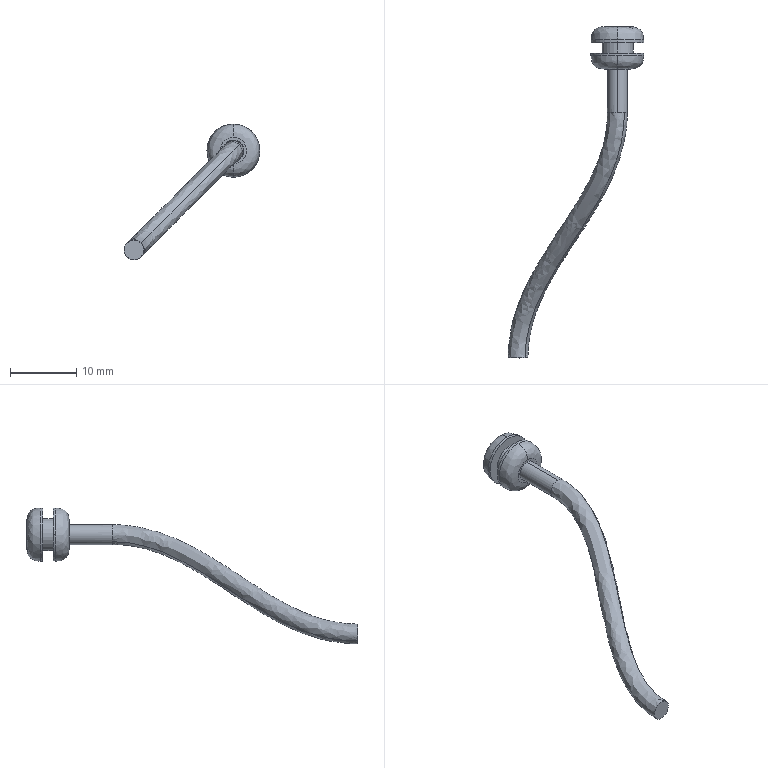Part | SolidWorks | features MirrorStock 1 | 2 solids | 22 faces | box 20.5 x 50.1 x 20.5 mm | volume 589.71 mm3 | cylinder 10 | plane 6 | spline 6 | commonest cylinder face diameters 8 x4 3 x2 3.2 x2 4.8 x2
STEP:
#1=CARTESIAN_POINT('',(0.,-64.8,-62.5));
#2=VERTEX_POINT('',#1);
#3=CARTESIAN_POINT('',(0.,-64.8,-59.5));
#4=VERTEX_POINT('',#3);
#5=CARTESIAN_POINT('',(0.,-64.8,-61.));
#6=DIRECTION('',(0.,1.,0.));
#7=DIRECTION('',(0.,0.,1.));
#8=AXIS2_PLACEMENT_3D('',#5,#6,#7);
#9=CIRCLE('',#8,1.5);
#10=EDGE_CURVE('',#2,#4,#9,.T.);
#11=ORIENTED_EDGE('',*,*,#10,.F.);
#12=CARTESIAN_POINT('',(0.,-77.8,-62.5));
#13=VERTEX_POINT('',#12);
#14=CARTESIAN_POINT('',(0.,-64.8,-62.5));
#15=DIRECTION('',(0.,-1.,0.));
#16=VECTOR('',#15,1000.);
#17=LINE('',#14,#16);
#18=EDGE_CURVE('',#2,#13,#17,.T.);
#19=ORIENTED_EDGE('',*,*,#18,.T.);
#20=CARTESIAN_POINT('',(-1.061,-77.8,-62.061));
#21=VERTEX_POINT('',#20);
#22=CARTESIAN_POINT('',(0.,-77.8,-62.5));
#23=CARTESIAN_POINT('',(-0.1963,-77.8,-62.5));
#24=CARTESIAN_POINT('',(-0.3926,-77.8,-62.461));
#25=CARTESIAN_POINT('',(-0.7554,-77.8,-62.311));
#26=CARTESIAN_POINT('',(-0.9218,-77.8,-62.2));
#27=CARTESIAN_POINT('',(-1.061,-77.8,-62.061));
#28=B_SPLINE_CURVE_WITH_KNOTS('',3,(#22,#23,#24,#25,#26,#27),.UNSPECIFIED.,.F.,.F.,(4,2,4),(0.6667,0.8333,1.),.UNSPECIFIED.);
#29=EDGE_CURVE('',#13,#21,#28,.T.);
#30=ORIENTED_EDGE('',*,*,#29,.T.);
#31=CARTESIAN_POINT('',(-1.5,-77.8,-61.));
#32=VERTEX_POINT('',#31);
#33=CARTESIAN_POINT('',(-1.061,-77.8,-62.061));
#34=CARTESIAN_POINT('',(-1.2,-77.8,-61.922));
#35=CARTESIAN_POINT('',(-1.311,-77.8,-61.755));
#36=CARTESIAN_POINT('',(-1.461,-77.8,-61.393));
#37=CARTESIAN_POINT('',(-1.5,-77.8,-61.196));
#38=CARTESIAN_POINT('',(-1.5,-77.8,-61.));
#39=B_SPLINE_CURVE_WITH_KNOTS('',3,(#33,#34,#35,#36,#37,#38),.UNSPECIFIED.,.F.,.F.,(4,2,4),(0.,0.5,1.),.UNSPECIFIED.);
#40=EDGE_CURVE('',#21,#32,#39,.T.);
#41=ORIENTED_EDGE('',*,*,#40,.T.);
#42=CARTESIAN_POINT('',(0.,-77.8,-59.5));
#43=VERTEX_POINT('',#42);
#44=CARTESIAN_POINT('',(-1.5,-77.8,-61.));
#45=CARTESIAN_POINT('',(-1.5,-77.8,-60.804));
#46=CARTESIAN_POINT('',(-1.461,-77.8,-60.607));
#47=CARTESIAN_POINT('',(-1.311,-77.8,-60.245));
#48=CARTESIAN_POINT('',(-1.2,-77.8,-60.078));
#49=CARTESIAN_POINT('',(-0.9218,-77.8,-59.8));
#50=CARTESIAN_POINT('',(-0.7554,-77.8,-59.689));
#51=CARTESIAN_POINT('',(-0.3926,-77.8,-59.539));
#52=CARTESIAN_POINT('',(-0.1963,-77.8,-59.5));
#53=CARTESIAN_POINT('',(0.,-77.8,-59.5));
#54=B_SPLINE_CURVE_WITH_KNOTS('',3,(#44,#45,#46,#47,#48,#49,#50,#51,#52,#53),.UNSPECIFIED.,.F.,.F.,(4,2,2,2,4),(0.,0.1667,0.3333,0.5,0.6667),.UNSPECIFIED.);
#55=EDGE_CURVE('',#32,#43,#54,.T.);
#56=ORIENTED_EDGE('',*,*,#55,.T.);
#57=CARTESIAN_POINT('',(0.,-64.8,-59.5));
#58=DIRECTION('',(0.,-1.,0.));
#59=VECTOR('',#58,1000.);
#60=LINE('',#57,#59);
#61=EDGE_CURVE('',#4,#43,#60,.T.);
#62=ORIENTED_EDGE('',*,*,#61,.F.);
#63=EDGE_LOOP('',(#11,#19,#30,#41,#56,#62));
#64=FACE_OUTER_BOUND('',#63,.T.);
#65=CARTESIAN_POINT('',(0.,-64.8,-61.));
#66=DIRECTION('',(0.,-1.,0.));
#67=DIRECTION('',(0.,0.,1.));
#68=AXIS2_PLACEMENT_3D('',#65,#66,#67);
#69=CYLINDRICAL_SURFACE('',#68,1.5);
#70=ADVANCED_FACE('',(#64),#69,.T.);
#71=CARTESIAN_POINT('',(-16.061,-114.9,-77.061));
#72=VERTEX_POINT('',#71);
#73=CARTESIAN_POINT('',(-13.939,-114.9,-74.939));
#74=VERTEX_POINT('',#73);
#75=CARTESIAN_POINT('',(-16.061,-114.9,-77.061));
#76=CARTESIAN_POINT('',(-15.784,-114.9,-77.338));
#77=CARTESIAN_POINT('',(-15.,-114.9,-77.662));
#78=CARTESIAN_POINT('',(-13.825,-114.9,-77.175));
#79=CARTESIAN_POINT('',(-13.338,-114.9,-76.));
#80=CARTESIAN_POINT('',(-13.662,-114.9,-75.216));
#81=CARTESIAN_POINT('',(-13.939,-114.9,-74.939));
#82=B_SPLINE_CURVE_WITH_KNOTS('',3,(#75,#76,#77,#78,#79,#80,#81),.UNSPECIFIED.,.F.,.F.,(4,1,1,1,4),(0.,0.001171,0.002343,0.003514,0.004685),.UNSPECIFIED.);
#83=EDGE_CURVE('',#72,#74,#82,.T.);
#84=ORIENTED_EDGE('',*,*,#83,.T.);
#85=CARTESIAN_POINT('',(-13.939,-114.9,-74.939));
#86=CARTESIAN_POINT('',(-14.216,-114.9,-74.662));
#87=CARTESIAN_POINT('',(-15.,-114.9,-74.338));
#88=CARTESIAN_POINT('',(-16.175,-114.9,-74.825));
#89=CARTESIAN_POINT('',(-16.662,-114.9,-76.));
#90=CARTESIAN_POINT('',(-16.338,-114.9,-76.784));
#91=CARTESIAN_POINT('',(-16.061,-114.9,-77.061));
#92=B_SPLINE_CURVE_WITH_KNOTS('',3,(#85,#86,#87,#88,#89,#90,#91),.UNSPECIFIED.,.F.,.F.,(4,1,1,1,4),(0.,0.001171,0.002343,0.003514,0.004685),.UNSPECIFIED.);
#93=EDGE_CURVE('',#74,#72,#92,.T.);
#94=ORIENTED_EDGE('',*,*,#93,.T.);
#95=EDGE_LOOP('',(#84,#94));
#96=FACE_OUTER_BOUND('',#95,.T.);
#97=CARTESIAN_POINT('',(-17.247,-114.9,-75.997));
#98=DIRECTION('',(0.,-1.,0.));
#99=DIRECTION('',(0.7071,0.,0.7071));
#100=AXIS2_PLACEMENT_3D('',#97,#98,#99);
#101=PLANE('',#100);
#102=ADVANCED_FACE('',(#96),#101,.T.);
#103=ORIENTED_EDGE('',*,*,#93,.F.);
#104=CARTESIAN_POINT('',(1.061,-77.8,-59.939));
#105=VERTEX_POINT('',#104);
#106=CARTESIAN_POINT('',(-13.939,-114.9,-74.939));
#107=CARTESIAN_POINT('',(-13.939,-113.106,-74.939));
#108=CARTESIAN_POINT('',(-13.435,-109.847,-74.435));
#109=CARTESIAN_POINT('',(-11.557,-105.198,-72.557));
#110=CARTESIAN_POINT('',(-9.047,-100.887,-70.047));
#111=CARTESIAN_POINT('',(-6.197,-96.586,-67.197));
#112=CARTESIAN_POINT('',(-3.422,-92.297,-64.422));
#113=CARTESIAN_POINT('',(-1.007,-87.743,-62.007));
#114=CARTESIAN_POINT('',(0.6349,-83.009,-60.365));
#115=CARTESIAN_POINT('',(1.061,-79.54,-59.939));
#116=CARTESIAN_POINT('',(1.061,-77.8,-59.939));
#117=B_SPLINE_CURVE_WITH_KNOTS('',3,(#106,#107,#108,#109,#110,#111,#112,#113,#114,#115,#116),.UNSPECIFIED.,.F.,.F.,(4,1,1,1,1,1,1,1,4),(0.002889,6.012,11.559,17.106,22.226,27.773,32.893,38.013,42.739),.UNSPECIFIED.);
#118=EDGE_CURVE('',#74,#105,#117,.T.);
#119=ORIENTED_EDGE('',*,*,#118,.T.);
#120=CARTESIAN_POINT('',(0.,-77.8,-59.5));
#121=CARTESIAN_POINT('',(0.1963,-77.8,-59.5));
#122=CARTESIAN_POINT('',(0.3926,-77.8,-59.539));
#123=CARTESIAN_POINT('',(0.7554,-77.8,-59.689));
#124=CARTESIAN_POINT('',(0.9218,-77.8,-59.8));
#125=CARTESIAN_POINT('',(1.061,-77.8,-59.939));
#126=B_SPLINE_CURVE_WITH_KNOTS('',3,(#120,#121,#122,#123,#124,#125),.UNSPECIFIED.,.F.,.F.,(4,2,4),(0.6667,0.8333,1.),.UNSPECIFIED.);
#127=EDGE_CURVE('',#43,#105,#126,.T.);
#128=ORIENTED_EDGE('',*,*,#127,.F.);
#129=ORIENTED_EDGE('',*,*,#55,.F.);
#130=ORIENTED_EDGE('',*,*,#40,.F.);
#131=CARTESIAN_POINT('',(-1.061,-77.8,-62.061));
#132=CARTESIAN_POINT('',(-1.061,-79.211,-62.061));
#133=CARTESIAN_POINT('',(-1.399,-82.018,-62.399));
#134=CARTESIAN_POINT('',(-2.804,-86.118,-63.804));
#135=CARTESIAN_POINT('',(-5.035,-90.343,-66.035));
#136=CARTESIAN_POINT('',(-7.735,-94.521,-68.735));
#137=CARTESIAN_POINT('',(-10.622,-98.874,-71.622));
#138=CARTESIAN_POINT('',(-13.281,-103.43,-74.281));
#139=CARTESIAN_POINT('',(-15.424,-108.672,-76.424));
#140=CARTESIAN_POINT('',(-16.061,-112.688,-77.061));
#141=CARTESIAN_POINT('',(-16.061,-114.9,-77.061));
#142=B_SPLINE_CURVE_WITH_KNOTS('',3,(#131,#132,#133,#134,#135,#136,#137,#138,#139,#140,#141),.UNSPECIFIED.,.F.,.F.,(4,1,1,1,1,1,1,1,4),(0.,4.726,9.846,14.967,20.514,25.634,31.181,36.727,42.737),.UNSPECIFIED.);
#143=EDGE_CURVE('',#21,#72,#142,.T.);
#144=ORIENTED_EDGE('',*,*,#143,.T.);
#145=EDGE_LOOP('',(#103,#119,#128,#129,#130,#144));
#146=FACE_OUTER_BOUND('',#145,.T.);
#147=CARTESIAN_POINT('',(-0.9955,-77.445,-62.128));
#148=CARTESIAN_POINT('',(-0.9658,-78.985,-62.099));
#149=CARTESIAN_POINT('',(-1.294,-81.911,-62.427));
#150=CARTESIAN_POINT('',(-2.736,-86.119,-63.869));
#151=CARTESIAN_POINT('',(-4.967,-90.345,-66.1));
#152=CARTESIAN_POINT('',(-7.667,-94.523,-68.8));
#153=CARTESIAN_POINT('',(-10.553,-98.876,-71.686));
#154=CARTESIAN_POINT('',(-13.212,-103.431,-74.345));
#155=CARTESIAN_POINT('',(-15.406,-108.795,-76.539));
#156=CARTESIAN_POINT('',(-16.035,-112.965,-77.168));
#157=CARTESIAN_POINT('',(-15.988,-115.341,-77.121));
#158=CARTESIAN_POINT('',(-1.019,-77.445,-62.108));
#159=CARTESIAN_POINT('',(-0.9894,-78.985,-62.078));
#160=CARTESIAN_POINT('',(-1.317,-81.911,-62.406));
#161=CARTESIAN_POINT('',(-2.759,-86.118,-63.848));
#162=CARTESIAN_POINT('',(-4.991,-90.344,-66.079));
#163=CARTESIAN_POINT('',(-7.69,-94.522,-68.779));
#164=CARTESIAN_POINT('',(-10.577,-98.875,-71.665));
#165=CARTESIAN_POINT('',(-13.236,-103.43,-74.324));
#166=CARTESIAN_POINT('',(-15.429,-108.794,-76.518));
#167=CARTESIAN_POINT('',(-16.058,-112.965,-77.147));
#168=CARTESIAN_POINT('',(-16.011,-115.341,-77.1));
#169=CARTESIAN_POINT('',(-1.328,-77.445,-61.818));
#170=CARTESIAN_POINT('',(-1.299,-78.984,-61.789));
#171=CARTESIAN_POINT('',(-1.626,-81.906,-62.116));
#172=CARTESIAN_POINT('',(-3.067,-86.111,-63.557));
#173=CARTESIAN_POINT('',(-5.297,-90.334,-65.788));
#174=CARTESIAN_POINT('',(-7.997,-94.512,-68.487));
#175=CARTESIAN_POINT('',(-10.883,-98.865,-71.373));
#176=CARTESIAN_POINT('',(-13.543,-103.422,-74.033));
#177=CARTESIAN_POINT('',(-15.738,-108.789,-76.228));
#178=CARTESIAN_POINT('',(-16.368,-112.963,-76.858));
#179=CARTESIAN_POINT('',(-16.32,-115.342,-76.811));
#180=CARTESIAN_POINT('',(-1.666,-77.436,-61.004));
#181=CARTESIAN_POINT('',(-1.635,-79.015,-60.973));
#182=CARTESIAN_POINT('',(-1.973,-82.016,-61.31));
#183=CARTESIAN_POINT('',(-3.441,-86.293,-62.779));
#184=CARTESIAN_POINT('',(-5.692,-90.554,-65.03));
#185=CARTESIAN_POINT('',(-8.4,-94.744,-67.738));
#186=CARTESIAN_POINT('',(-11.282,-99.092,-70.62));
#187=CARTESIAN_POINT('',(-13.925,-103.621,-73.263));
#188=CARTESIAN_POINT('',(-16.089,-108.919,-75.427));
#189=CARTESIAN_POINT('',(-16.704,-113.004,-76.042));
#190=CARTESIAN_POINT('',(-16.658,-115.332,-75.996));
#191=CARTESIAN_POINT('',(-1.179,-77.403,-59.828));
#192=CARTESIAN_POINT('',(-1.146,-79.123,-59.795));
#193=CARTESIAN_POINT('',(-1.517,-82.397,-60.167));
#194=CARTESIAN_POINT('',(-3.081,-86.93,-61.73));
#195=CARTESIAN_POINT('',(-5.404,-91.32,-64.053));
#196=CARTESIAN_POINT('',(-8.142,-95.554,-66.791));
#197=CARTESIAN_POINT('',(-11.01,-99.881,-69.659));
#198=CARTESIAN_POINT('',(-13.594,-104.314,-72.244));
#199=CARTESIAN_POINT('',(-15.652,-109.374,-74.301));
#200=CARTESIAN_POINT('',(-16.214,-113.148,-74.863));
#201=CARTESIAN_POINT('',(-16.171,-115.3,-74.821));
#202=CARTESIAN_POINT('',(-0.004221,-77.371,-59.342));
#203=CARTESIAN_POINT('',(0.03237,-79.231,-59.305));
#204=CARTESIAN_POINT('',(-0.3736,-82.779,-59.711));
#205=CARTESIAN_POINT('',(-2.033,-87.567,-61.371));
#206=CARTESIAN_POINT('',(-4.428,-92.085,-63.766));
#207=CARTESIAN_POINT('',(-7.195,-96.363,-66.532));
#208=CARTESIAN_POINT('',(-10.049,-100.669,-69.386));
#209=CARTESIAN_POINT('',(-12.575,-105.007,-71.913));
#210=CARTESIAN_POINT('',(-14.526,-109.829,-73.864));
#211=CARTESIAN_POINT('',(-15.035,-113.291,-74.373));
#212=CARTESIAN_POINT('',(-14.996,-115.267,-74.334));
#213=CARTESIAN_POINT('',(0.8106,-77.362,-59.68));
#214=CARTESIAN_POINT('',(0.8481,-79.262,-59.642));
#215=CARTESIAN_POINT('',(0.4322,-82.889,-60.058));
#216=CARTESIAN_POINT('',(-1.255,-87.75,-61.745));
#217=CARTESIAN_POINT('',(-3.67,-92.305,-64.16));
#218=CARTESIAN_POINT('',(-6.445,-96.595,-66.936));
#219=CARTESIAN_POINT('',(-9.295,-100.896,-69.785));
#220=CARTESIAN_POINT('',(-11.805,-105.206,-72.295));
#221=CARTESIAN_POINT('',(-13.725,-109.96,-74.215));
#222=CARTESIAN_POINT('',(-14.219,-113.333,-74.709));
#223=CARTESIAN_POINT('',(-14.182,-115.257,-74.672));
#224=CARTESIAN_POINT('',(1.1,-77.362,-59.989));
#225=CARTESIAN_POINT('',(1.137,-79.261,-59.951));
#226=CARTESIAN_POINT('',(0.7219,-82.884,-60.367));
#227=CARTESIAN_POINT('',(-0.9638,-87.743,-62.052));
#228=CARTESIAN_POINT('',(-3.378,-92.296,-64.467));
#229=CARTESIAN_POINT('',(-6.153,-96.586,-67.242));
#230=CARTESIAN_POINT('',(-9.003,-100.886,-70.092));
#231=CARTESIAN_POINT('',(-11.514,-105.198,-72.602));
#232=CARTESIAN_POINT('',(-13.435,-109.955,-74.524));
#233=CARTESIAN_POINT('',(-13.93,-113.331,-75.018));
#234=CARTESIAN_POINT('',(-13.892,-115.258,-74.981));
#235=CARTESIAN_POINT('',(1.121,-77.362,-60.012));
#236=CARTESIAN_POINT('',(1.158,-79.261,-59.975));
#237=CARTESIAN_POINT('',(0.7426,-82.884,-60.39));
#238=CARTESIAN_POINT('',(-0.9429,-87.741,-62.076));
#239=CARTESIAN_POINT('',(-3.357,-92.295,-64.49));
#240=CARTESIAN_POINT('',(-6.132,-96.584,-67.265));
#241=CARTESIAN_POINT('',(-8.982,-100.885,-70.115));
#242=CARTESIAN_POINT('',(-11.493,-105.196,-72.626));
#243=CARTESIAN_POINT('',(-13.414,-109.954,-74.547));
#244=CARTESIAN_POINT('',(-13.909,-113.331,-75.042));
#245=CARTESIAN_POINT('',(-13.872,-115.258,-75.005));
#246=B_SPLINE_SURFACE_WITH_KNOTS('',3,3,((#147,#148,#149,#150,#151,#152,#153,#154,#155,#156,#157),(#158,#159,#160,#161,#162,#163,#164,#165,#166,#167,#168),(#169,#170,#171,#172,#173,#174,#175,#176,#177,#178,#179),(#180,#181,#182,#183,#184,#185,#186,#187,#188,#189,#190),(#191,#192,#193,#194,#195,#196,#197,#198,#199,#200,#201),(#202,#203,#204,#205,#206,#207,#208,#209,#210,#211,#212),(#213,#214,#215,#216,#217,#218,#219,#220,#221,#222,#223),(#224,#225,#226,#227,#228,#229,#230,#231,#232,#233,#234),(#235,#236,#237,#238,#239,#240,#241,#242,#243,#244,#245)),.UNSPECIFIED.,.F.,.F.,.F.,(4,1,1,1,1,1,4),(4,1,1,1,1,1,1,1,4),(0.49,0.5,0.625,0.75,0.875,1.,1.01),(-0.3952,4.726,9.846,14.967,20.514,25.634,31.181,36.727,43.135),.UNSPECIFIED.);
#247=ADVANCED_FACE('',(#146),#246,.F.);
#248=ORIENTED_EDGE('',*,*,#83,.F.);
#249=ORIENTED_EDGE('',*,*,#143,.F.);
#250=ORIENTED_EDGE('',*,*,#29,.F.);
#251=CARTESIAN_POINT('',(1.5,-77.8,-61.));
#252=VERTEX_POINT('',#251);
#253=CARTESIAN_POINT('',(1.5,-77.8,-61.));
#254=CARTESIAN_POINT('',(1.5,-77.8,-61.196));
#255=CARTESIAN_POINT('',(1.461,-77.8,-61.393));
#256=CARTESIAN_POINT('',(1.311,-77.8,-61.755));
#257=CARTESIAN_POINT('',(1.2,-77.8,-61.922));
#258=CARTESIAN_POINT('',(0.9218,-77.8,-62.2));
#259=CARTESIAN_POINT('',(0.7554,-77.8,-62.311));
#260=CARTESIAN_POINT('',(0.3926,-77.8,-62.461));
#261=CARTESIAN_POINT('',(0.1963,-77.8,-62.5));
#262=CARTESIAN_POINT('',(0.,-77.8,-62.5));
#263=B_SPLINE_CURVE_WITH_KNOTS('',3,(#253,#254,#255,#256,#257,#258,#259,#260,#261,#262),.UNSPECIFIED.,.F.,.F.,(4,2,2,2,4),(0.,0.1667,0.3333,0.5,0.6667),.UNSPECIFIED.);
#264=EDGE_CURVE('',#252,#13,#263,.T.);
#265=ORIENTED_EDGE('',*,*,#264,.F.);
#266=CARTESIAN_POINT('',(1.061,-77.8,-59.939));
#267=CARTESIAN_POINT('',(1.2,-77.8,-60.078));
#268=CARTESIAN_POINT('',(1.311,-77.8,-60.245));
#269=CARTESIAN_POINT('',(1.461,-77.8,-60.607));
#270=CARTESIAN_POINT('',(1.5,-77.8,-60.804));
#271=CARTESIAN_POINT('',(1.5,-77.8,-61.));
#272=B_SPLINE_CURVE_WITH_KNOTS('',3,(#266,#267,#268,#269,#270,#271),.UNSPECIFIED.,.F.,.F.,(4,2,4),(0.,0.5,1.),.UNSPECIFIED.);
#273=EDGE_CURVE('',#105,#252,#272,.T.);
#274=ORIENTED_EDGE('',*,*,#273,.F.);
#275=ORIENTED_EDGE('',*,*,#118,.F.);
#276=EDGE_LOOP('',(#248,#249,#250,#265,#274,#275));
#277=FACE_OUTER_BOUND('',#276,.T.);
#278=CARTESIAN_POINT('',(0.9877,-77.362,-59.879));
#279=CARTESIAN_POINT('',(1.025,-79.261,-59.842));
#280=CARTESIAN_POINT('',(0.6097,-82.884,-60.257));
#281=CARTESIAN_POINT('',(-1.076,-87.741,-61.943));
#282=CARTESIAN_POINT('',(-3.49,-92.295,-64.357));
#283=CARTESIAN_POINT('',(-6.265,-96.584,-67.132));
#284=CARTESIAN_POINT('',(-9.115,-100.885,-69.982));
#285=CARTESIAN_POINT('',(-11.626,-105.196,-72.493));
#286=CARTESIAN_POINT('',(-13.547,-109.954,-74.414));
#287=CARTESIAN_POINT('',(-14.042,-113.331,-74.909));
#288=CARTESIAN_POINT('',(-14.005,-115.258,-74.872));
#289=CARTESIAN_POINT('',(1.011,-77.362,-59.9));
#290=CARTESIAN_POINT('',(1.049,-79.261,-59.863));
#291=CARTESIAN_POINT('',(0.6332,-82.884,-60.278));
#292=CARTESIAN_POINT('',(-1.052,-87.743,-61.964));
#293=CARTESIAN_POINT('',(-3.467,-92.296,-64.378));
#294=CARTESIAN_POINT('',(-6.242,-96.586,-67.153));
#295=CARTESIAN_POINT('',(-9.092,-100.886,-70.003));
#296=CARTESIAN_POINT('',(-11.602,-105.198,-72.514));
#297=CARTESIAN_POINT('',(-13.524,-109.955,-74.435));
#298=CARTESIAN_POINT('',(-14.018,-113.331,-74.93));
#299=CARTESIAN_POINT('',(-13.981,-115.258,-74.892));
#300=CARTESIAN_POINT('',(1.32,-77.362,-60.189));
#301=CARTESIAN_POINT('',(1.358,-79.262,-60.152));
#302=CARTESIAN_POINT('',(0.942,-82.889,-60.568));
#303=CARTESIAN_POINT('',(-0.7448,-87.75,-62.255));
#304=CARTESIAN_POINT('',(-3.16,-92.305,-64.67));
#305=CARTESIAN_POINT('',(-5.936,-96.595,-67.445));
#306=CARTESIAN_POINT('',(-8.785,-100.896,-70.295));
#307=CARTESIAN_POINT('',(-11.295,-105.206,-72.805));
#308=CARTESIAN_POINT('',(-13.215,-109.96,-74.725));
#309=CARTESIAN_POINT('',(-13.709,-113.333,-75.219));
#310=CARTESIAN_POINT('',(-13.672,-115.257,-75.182));
#311=CARTESIAN_POINT('',(1.658,-77.371,-61.004));
#312=CARTESIAN_POINT('',(1.695,-79.231,-60.968));
#313=CARTESIAN_POINT('',(1.289,-82.779,-61.374));
#314=CARTESIAN_POINT('',(-0.3707,-87.567,-63.033));
#315=CARTESIAN_POINT('',(-2.766,-92.085,-65.428));
#316=CARTESIAN_POINT('',(-5.532,-96.363,-68.195));
#317=CARTESIAN_POINT('',(-8.386,-100.669,-71.049));
#318=CARTESIAN_POINT('',(-10.913,-105.007,-73.575));
#319=CARTESIAN_POINT('',(-12.864,-109.829,-75.526));
#320=CARTESIAN_POINT('',(-13.373,-113.291,-76.035));
#321=CARTESIAN_POINT('',(-13.334,-115.267,-75.996));
#322=CARTESIAN_POINT('',(1.172,-77.403,-62.179));
#323=CARTESIAN_POINT('',(1.205,-79.123,-62.146));
#324=CARTESIAN_POINT('',(0.8334,-82.397,-62.517));
#325=CARTESIAN_POINT('',(-0.7304,-86.93,-64.081));
#326=CARTESIAN_POINT('',(-3.053,-91.32,-66.404));
#327=CARTESIAN_POINT('',(-5.791,-95.554,-69.142));
#328=CARTESIAN_POINT('',(-8.659,-99.881,-72.01));
#329=CARTESIAN_POINT('',(-11.244,-104.314,-74.594));
#330=CARTESIAN_POINT('',(-13.301,-109.374,-76.652));
#331=CARTESIAN_POINT('',(-13.863,-113.148,-77.214));
#332=CARTESIAN_POINT('',(-13.821,-115.3,-77.171));
#333=CARTESIAN_POINT('',(-0.003522,-77.436,-62.666));
#334=CARTESIAN_POINT('',(0.02698,-79.015,-62.635));
#335=CARTESIAN_POINT('',(-0.3103,-82.016,-62.973));
#336=CARTESIAN_POINT('',(-1.779,-86.293,-64.441));
#337=CARTESIAN_POINT('',(-4.03,-90.554,-66.692));
#338=CARTESIAN_POINT('',(-6.738,-94.744,-69.4));
#339=CARTESIAN_POINT('',(-9.62,-99.092,-72.282));
#340=CARTESIAN_POINT('',(-12.263,-103.621,-74.925));
#341=CARTESIAN_POINT('',(-14.427,-108.919,-77.089));
#342=CARTESIAN_POINT('',(-15.042,-113.004,-77.704));
#343=CARTESIAN_POINT('',(-14.996,-115.332,-77.658));
#344=CARTESIAN_POINT('',(-0.8184,-77.445,-62.328));
#345=CARTESIAN_POINT('',(-0.7887,-78.984,-62.299));
#346=CARTESIAN_POINT('',(-1.116,-81.906,-62.626));
#347=CARTESIAN_POINT('',(-2.557,-86.111,-64.067));
#348=CARTESIAN_POINT('',(-4.788,-90.334,-66.297));
#349=CARTESIAN_POINT('',(-7.487,-94.512,-68.997));
#350=CARTESIAN_POINT('',(-10.373,-98.865,-71.883));
#351=CARTESIAN_POINT('',(-13.033,-103.422,-74.543));
#352=CARTESIAN_POINT('',(-15.228,-108.789,-76.738));
#353=CARTESIAN_POINT('',(-15.858,-112.963,-77.368));
#354=CARTESIAN_POINT('',(-15.811,-115.342,-77.32));
#355=CARTESIAN_POINT('',(-1.108,-77.445,-62.019));
#356=CARTESIAN_POINT('',(-1.078,-78.985,-61.989));
#357=CARTESIAN_POINT('',(-1.406,-81.911,-62.317));
#358=CARTESIAN_POINT('',(-2.848,-86.118,-63.759));
#359=CARTESIAN_POINT('',(-5.079,-90.344,-65.991));
#360=CARTESIAN_POINT('',(-7.779,-94.522,-68.69));
#361=CARTESIAN_POINT('',(-10.665,-98.875,-71.577));
#362=CARTESIAN_POINT('',(-13.324,-103.43,-74.236));
#363=CARTESIAN_POINT('',(-15.518,-108.794,-76.429));
#364=CARTESIAN_POINT('',(-16.147,-112.965,-77.058));
#365=CARTESIAN_POINT('',(-16.1,-115.341,-77.011));
#366=CARTESIAN_POINT('',(-1.128,-77.445,-61.995));
#367=CARTESIAN_POINT('',(-1.099,-78.985,-61.966));
#368=CARTESIAN_POINT('',(-1.427,-81.911,-62.294));
#369=CARTESIAN_POINT('',(-2.869,-86.119,-63.736));
#370=CARTESIAN_POINT('',(-5.1,-90.345,-65.967));
#371=CARTESIAN_POINT('',(-7.8,-94.523,-68.667));
#372=CARTESIAN_POINT('',(-10.686,-98.876,-71.553));
#373=CARTESIAN_POINT('',(-13.345,-103.431,-74.212));
#374=CARTESIAN_POINT('',(-15.539,-108.795,-76.406));
#375=CARTESIAN_POINT('',(-16.168,-112.965,-77.035));
#376=CARTESIAN_POINT('',(-16.121,-115.341,-76.988));
#377=B_SPLINE_SURFACE_WITH_KNOTS('',3,3,((#278,#279,#280,#281,#282,#283,#284,#285,#286,#287,#288),(#289,#290,#291,#292,#293,#294,#295,#296,#297,#298,#299),(#300,#301,#302,#303,#304,#305,#306,#307,#308,#309,#310),(#311,#312,#313,#314,#315,#316,#317,#318,#319,#320,#321),(#322,#323,#324,#325,#326,#327,#328,#329,#330,#331,#332),(#333,#334,#335,#336,#337,#338,#339,#340,#341,#342,#343),(#344,#345,#346,#347,#348,#349,#350,#351,#352,#353,#354),(#355,#356,#357,#358,#359,#360,#361,#362,#363,#364,#365),(#366,#367,#368,#369,#370,#371,#372,#373,#374,#375,#376)),.UNSPECIFIED.,.F.,.F.,.F.,(4,1,1,1,1,1,4),(4,1,1,1,1,1,1,1,4),(-0.01,0.,0.125,0.25,0.375,0.5,0.51),(-0.3952,4.726,9.846,14.967,20.514,25.634,31.181,36.727,43.135),.UNSPECIFIED.);
#378=ADVANCED_FACE('',(#277),#377,.F.);
#379=ORIENTED_EDGE('',*,*,#18,.F.);
#380=CARTESIAN_POINT('',(0.,-64.8,-61.));
#381=DIRECTION('',(0.,1.,0.));
#382=DIRECTION('',(0.,0.,1.));
#383=AXIS2_PLACEMENT_3D('',#380,#381,#382);
#384=CIRCLE('',#383,1.5);
#385=EDGE_CURVE('',#4,#2,#384,.T.);
#386=ORIENTED_EDGE('',*,*,#385,.F.);
#387=ORIENTED_EDGE('',*,*,#61,.T.);
#388=ORIENTED_EDGE('',*,*,#127,.T.);
#389=ORIENTED_EDGE('',*,*,#273,.T.);
#390=ORIENTED_EDGE('',*,*,#264,.T.);
#391=EDGE_LOOP('',(#379,#386,#387,#388,#389,#390));
#392=FACE_OUTER_BOUND('',#391,.T.);
#393=CARTESIAN_POINT('',(0.,-64.8,-61.));
#394=DIRECTION('',(0.,-1.,0.));
#395=DIRECTION('',(0.,0.,1.));
#396=AXIS2_PLACEMENT_3D('',#393,#394,#395);
#397=CYLINDRICAL_SURFACE('',#396,1.5);
#398=ADVANCED_FACE('',(#392),#397,.T.);
#399=ORIENTED_EDGE('',*,*,#385,.T.);
#400=ORIENTED_EDGE('',*,*,#10,.T.);
#401=EDGE_LOOP('',(#399,#400));
#402=FACE_OUTER_BOUND('',#401,.T.);
#403=CARTESIAN_POINT('',(1.587,-64.8,-62.589));
#404=DIRECTION('',(0.,-1.,0.));
#405=DIRECTION('',(-1.,0.,0.));
#406=AXIS2_PLACEMENT_3D('',#403,#404,#405);
#407=PLANE('',#406);
#408=ADVANCED_FACE('',(#402),#407,.F.);
#409=CLOSED_SHELL('',(#70,#102,#247,#378,#398,#408));
#410=MANIFOLD_SOLID_BREP('',#409);
#411=CARTESIAN_POINT('',(-0.0142,-64.9,-63.));
#412=VERTEX_POINT('',#411);
#413=CARTESIAN_POINT('',(0.,-64.9,-59.));
#414=VERTEX_POINT('',#413);
#415=CARTESIAN_POINT('',(-0.0142,-64.9,-63.));
#416=CARTESIAN_POINT('',(-0.2764,-64.9,-62.998));
#417=CARTESIAN_POINT('',(-0.5349,-64.9,-62.945));
#418=CARTESIAN_POINT('',(-1.019,-64.9,-62.741));
#419=CARTESIAN_POINT('',(-1.237,-64.9,-62.593));
#420=CARTESIAN_POINT('',(-1.606,-64.9,-62.22));
#421=CARTESIAN_POINT('',(-1.752,-64.9,-62.));
#422=CARTESIAN_POINT('',(-1.951,-64.9,-61.514));
#423=CARTESIAN_POINT('',(-2.001,-64.9,-61.256));
#424=CARTESIAN_POINT('',(-1.999,-64.9,-60.73));
#425=CARTESIAN_POINT('',(-1.947,-64.9,-60.472));
#426=CARTESIAN_POINT('',(-1.744,-64.9,-59.987));
#427=CARTESIAN_POINT('',(-1.598,-64.9,-59.769));
#428=CARTESIAN_POINT('',(-1.226,-64.9,-59.398));
#429=CARTESIAN_POINT('',(-1.007,-64.9,-59.252));
#430=CARTESIAN_POINT('',(-0.5209,-64.9,-59.051));
#431=CARTESIAN_POINT('',(-0.2617,-64.9,-59.));
#432=CARTESIAN_POINT('',(0.,-64.9,-59.));
#433=B_SPLINE_CURVE_WITH_KNOTS('',3,(#415,#416,#417,#418,#419,#420,#421,#422,#423,#424,#425,#426,#427,#428,#429,#430,#431,#432),.UNSPECIFIED.,.F.,.F.,(4,2,2,2,2,2,2,2,4),(0.00225,0.127,0.2517,0.3764,0.5011,0.6258,0.7506,0.8753,1.),.UNSPECIFIED.);
#434=EDGE_CURVE('',#412,#414,#433,.T.);
#435=ORIENTED_EDGE('',*,*,#434,.F.);
#436=CARTESIAN_POINT('',(-0.02839,-66.9,-65.));
#437=VERTEX_POINT('',#436);
#438=CARTESIAN_POINT('',(-0.0142,-64.9,-63.));
#439=CARTESIAN_POINT('',(-0.02366,-64.9,-64.333));
#440=CARTESIAN_POINT('',(-0.02839,-65.567,-65.));
#441=CARTESIAN_POINT('',(-0.02839,-66.9,-65.));
#442=B_SPLINE_CURVE_WITH_KNOTS('',3,(#438,#439,#440,#441),.UNSPECIFIED.,.F.,.F.,(4,4),(0.01056,0.9893),.UNSPECIFIED.);
#443=EDGE_CURVE('',#412,#437,#442,.T.);
#444=ORIENTED_EDGE('',*,*,#443,.T.);
#445=CARTESIAN_POINT('',(0.,-66.9,-57.));
#446=VERTEX_POINT('',#445);
#447=CARTESIAN_POINT('',(0.,-66.9,-61.));
#448=DIRECTION('',(0.,1.,0.));
#449=DIRECTION('',(0.007098,0.,1.));
#450=AXIS2_PLACEMENT_3D('',#447,#448,#449);
#451=CIRCLE('',#450,4.);
#452=EDGE_CURVE('',#437,#446,#451,.T.);
#453=ORIENTED_EDGE('',*,*,#452,.T.);
#454=CARTESIAN_POINT('',(0.02839,-66.9,-57.));
#455=VERTEX_POINT('',#454);
#456=CARTESIAN_POINT('',(0.,-66.9,-61.));
#457=DIRECTION('',(0.,1.,0.));
#458=DIRECTION('',(0.007098,0.,1.));
#459=AXIS2_PLACEMENT_3D('',#456,#457,#458);
#460=CIRCLE('',#459,4.);
#461=EDGE_CURVE('',#446,#455,#460,.T.);
#462=ORIENTED_EDGE('',*,*,#461,.T.);
#463=CARTESIAN_POINT('',(0.0142,-64.9,-59.));
#464=VERTEX_POINT('',#463);
#465=CARTESIAN_POINT('',(0.0142,-64.9,-59.));
#466=CARTESIAN_POINT('',(0.02366,-64.9,-57.667));
#467=CARTESIAN_POINT('',(0.02839,-65.567,-57.));
#468=CARTESIAN_POINT('',(0.02839,-66.9,-57.));
#469=B_SPLINE_CURVE_WITH_KNOTS('',3,(#465,#466,#467,#468),.UNSPECIFIED.,.F.,.F.,(4,4),(0.01056,0.9893),.UNSPECIFIED.);
#470=EDGE_CURVE('',#464,#455,#469,.T.);
#471=ORIENTED_EDGE('',*,*,#470,.F.);
#472=CARTESIAN_POINT('',(0.,-64.9,-59.));
#473=CARTESIAN_POINT('',(0.004734,-64.9,-59.));
#474=CARTESIAN_POINT('',(0.009466,-64.9,-59.));
#475=CARTESIAN_POINT('',(0.0142,-64.9,-59.));
#476=B_SPLINE_CURVE_WITH_KNOTS('',3,(#472,#473,#474,#475),.UNSPECIFIED.,.F.,.F.,(4,4),(0.,0.00225),.UNSPECIFIED.);
#477=EDGE_CURVE('',#414,#464,#476,.T.);
#478=ORIENTED_EDGE('',*,*,#477,.F.);
#479=EDGE_LOOP('',(#435,#444,#453,#462,#471,#478));
#480=FACE_OUTER_BOUND('',#479,.T.);
#481=CARTESIAN_POINT('',(0.0142,-64.9,-59.));
#482=CARTESIAN_POINT('',(-1.157,-64.9,-58.992));
#483=CARTESIAN_POINT('',(-1.992,-64.9,-59.814));
#484=CARTESIAN_POINT('',(-2.,-64.9,-60.986));
#485=CARTESIAN_POINT('',(-2.008,-64.9,-62.157));
#486=CARTESIAN_POINT('',(-1.186,-64.9,-62.992));
#487=CARTESIAN_POINT('',(-0.0142,-64.9,-63.));
#488=CARTESIAN_POINT('',(0.02366,-64.9,-57.667));
#489=CARTESIAN_POINT('',(-1.929,-64.9,-57.653));
#490=CARTESIAN_POINT('',(-3.319,-64.9,-59.024));
#491=CARTESIAN_POINT('',(-3.333,-64.9,-60.976));
#492=CARTESIAN_POINT('',(-3.347,-64.9,-62.929));
#493=CARTESIAN_POINT('',(-1.976,-64.9,-64.319));
#494=CARTESIAN_POINT('',(-0.02366,-64.9,-64.333));
#495=CARTESIAN_POINT('',(0.02839,-65.567,-57.));
#496=CARTESIAN_POINT('',(-2.315,-65.567,-56.983));
#497=CARTESIAN_POINT('',(-3.983,-65.567,-58.629));
#498=CARTESIAN_POINT('',(-4.,-65.567,-60.972));
#499=CARTESIAN_POINT('',(-4.017,-65.567,-63.315));
#500=CARTESIAN_POINT('',(-2.371,-65.567,-64.983));
#501=CARTESIAN_POINT('',(-0.02839,-65.567,-65.));
#502=CARTESIAN_POINT('',(0.02839,-66.9,-57.));
#503=CARTESIAN_POINT('',(-2.315,-66.9,-56.983));
#504=CARTESIAN_POINT('',(-3.983,-66.9,-58.629));
#505=CARTESIAN_POINT('',(-4.,-66.9,-60.972));
#506=CARTESIAN_POINT('',(-4.017,-66.9,-63.315));
#507=CARTESIAN_POINT('',(-2.371,-66.9,-64.983));
#508=CARTESIAN_POINT('',(-0.02839,-66.9,-65.));
#509=(BOUNDED_SURFACE()B_SPLINE_SURFACE(3,3,((#481,#482,#483,#484,#485,#486,#487),(#488,#489,#490,#491,#492,#493,#494),(#495,#496,#497,#498,#499,#500,#501),(#502,#503,#504,#505,#506,#507,#508)),.UNSPECIFIED.,.F.,.F.,.F.)B_SPLINE_SURFACE_WITH_KNOTS((4,4),(4,3,4),(0.01056,0.9893),(0.,0.5,1.),.UNSPECIFIED.)GEOMETRIC_REPRESENTATION_ITEM()RATIONAL_B_SPLINE_SURFACE(((1.,0.8047,0.8047,1.,0.8047,0.8047,1.),(1.,0.8047,0.8047,1.,0.8047,0.8047,1.),(1.,0.8047,0.8047,1.,0.8047,0.8047,1.),(1.,0.8047,0.8047,1.,0.8047,0.8047,1.)))REPRESENTATION_ITEM('')SURFACE());
#510=ADVANCED_FACE('',(#480),#509,.F.);
#511=CARTESIAN_POINT('',(4.,-69.3,-61.));
#512=VERTEX_POINT('',#511);
#513=CARTESIAN_POINT('',(-0.01999,-69.3,-57.));
#514=VERTEX_POINT('',#513);
#515=CARTESIAN_POINT('',(0.,-69.3,-61.));
#516=DIRECTION('',(0.,-1.,0.));
#517=DIRECTION('',(0.004997,0.,-1.));
#518=AXIS2_PLACEMENT_3D('',#515,#516,#517);
#519=CIRCLE('',#518,4.);
#520=EDGE_CURVE('',#512,#514,#519,.T.);
#521=ORIENTED_EDGE('',*,*,#520,.T.);
#522=CARTESIAN_POINT('',(-0.009993,-71.3,-59.));
#523=VERTEX_POINT('',#522);
#524=CARTESIAN_POINT('',(-0.01999,-69.3,-57.));
#525=CARTESIAN_POINT('',(-0.01999,-70.633,-57.));
#526=CARTESIAN_POINT('',(-0.01666,-71.3,-57.667));
#527=CARTESIAN_POINT('',(-0.009993,-71.3,-59.));
#528=B_SPLINE_CURVE_WITH_KNOTS('',3,(#524,#525,#526,#527),.UNSPECIFIED.,.F.,.F.,(4,4),(0.01056,0.9893),.UNSPECIFIED.);
#529=EDGE_CURVE('',#514,#523,#528,.T.);
#530=ORIENTED_EDGE('',*,*,#529,.T.);
#531=CARTESIAN_POINT('',(0.,-71.3,-59.));
#532=VERTEX_POINT('',#531);
#533=CARTESIAN_POINT('',(-0.009993,-71.3,-59.));
#534=CARTESIAN_POINT('',(-0.006662,-71.3,-59.));
#535=CARTESIAN_POINT('',(-0.003331,-71.3,-59.));
#536=CARTESIAN_POINT('',(0.,-71.3,-59.));
#537=(BOUNDED_CURVE()B_SPLINE_CURVE(3,(#533,#534,#535,#536),.UNSPECIFIED.,.F.,.T.)B_SPLINE_CURVE_WITH_KNOTS((4,4),(0.9984,1.),.UNSPECIFIED.)CURVE()GEOMETRIC_REPRESENTATION_ITEM()RATIONAL_B_SPLINE_CURVE((1.,1.,1.,1.))REPRESENTATION_ITEM(''));
#538=EDGE_CURVE('',#523,#532,#537,.T.);
#539=ORIENTED_EDGE('',*,*,#538,.T.);
#540=CARTESIAN_POINT('',(0.009993,-71.3,-63.));
#541=VERTEX_POINT('',#540);
#542=CARTESIAN_POINT('',(0.,-71.3,-59.));
#543=CARTESIAN_POINT('',(3.98,-71.3,-59.));
#544=CARTESIAN_POINT('',(3.99,-71.3,-62.98));
#545=CARTESIAN_POINT('',(0.009993,-71.3,-63.));
#546=(BOUNDED_CURVE()B_SPLINE_CURVE(3,(#542,#543,#544,#545),.UNSPECIFIED.,.F.,.T.)B_SPLINE_CURVE_WITH_KNOTS((4,4),(0.,0.9984),.UNSPECIFIED.)CURVE()GEOMETRIC_REPRESENTATION_ITEM()RATIONAL_B_SPLINE_CURVE((1.,0.335,0.335,1.))REPRESENTATION_ITEM(''));
#547=EDGE_CURVE('',#532,#541,#546,.T.);
#548=ORIENTED_EDGE('',*,*,#547,.T.);
#549=CARTESIAN_POINT('',(0.01999,-69.3,-65.));
#550=VERTEX_POINT('',#549);
#551=CARTESIAN_POINT('',(0.01999,-69.3,-65.));
#552=CARTESIAN_POINT('',(0.01999,-70.633,-65.));
#553=CARTESIAN_POINT('',(0.01666,-71.3,-64.333));
#554=CARTESIAN_POINT('',(0.009993,-71.3,-63.));
#555=B_SPLINE_CURVE_WITH_KNOTS('',3,(#551,#552,#553,#554),.UNSPECIFIED.,.F.,.F.,(4,4),(0.01056,0.9893),.UNSPECIFIED.);
#556=EDGE_CURVE('',#550,#541,#555,.T.);
#557=ORIENTED_EDGE('',*,*,#556,.F.);
#558=CARTESIAN_POINT('',(0.,-69.3,-61.));
#559=DIRECTION('',(0.,-1.,0.));
#560=DIRECTION('',(0.004997,0.,-1.));
#561=AXIS2_PLACEMENT_3D('',#558,#559,#560);
#562=CIRCLE('',#561,4.);
#563=EDGE_CURVE('',#550,#512,#562,.T.);
#564=ORIENTED_EDGE('',*,*,#563,.T.);
#565=EDGE_LOOP('',(#521,#530,#539,#548,#557,#564));
#566=FACE_OUTER_BOUND('',#565,.T.);
#567=CARTESIAN_POINT('',(0.01999,-69.3,-65.));
#568=CARTESIAN_POINT('',(8.02,-69.3,-64.96));
#569=CARTESIAN_POINT('',(7.98,-69.3,-56.96));
#570=CARTESIAN_POINT('',(-0.01999,-69.3,-57.));
#571=CARTESIAN_POINT('',(0.01999,-70.633,-65.));
#572=CARTESIAN_POINT('',(8.02,-70.633,-64.96));
#573=CARTESIAN_POINT('',(7.98,-70.633,-56.96));
#574=CARTESIAN_POINT('',(-0.01999,-70.633,-57.));
#575=CARTESIAN_POINT('',(0.01666,-71.3,-64.333));
#576=CARTESIAN_POINT('',(6.683,-71.3,-64.3));
#577=CARTESIAN_POINT('',(6.65,-71.3,-57.633));
#578=CARTESIAN_POINT('',(-0.01666,-71.3,-57.667));
#579=CARTESIAN_POINT('',(0.009993,-71.3,-63.));
#580=CARTESIAN_POINT('',(4.01,-71.3,-62.98));
#581=CARTESIAN_POINT('',(3.99,-71.3,-58.98));
#582=CARTESIAN_POINT('',(-0.009993,-71.3,-59.));
#583=(BOUNDED_SURFACE()B_SPLINE_SURFACE(3,3,((#567,#568,#569,#570),(#571,#572,#573,#574),(#575,#576,#577,#578),(#579,#580,#581,#582)),.UNSPECIFIED.,.F.,.F.,.F.)B_SPLINE_SURFACE_WITH_KNOTS((4,4),(4,4),(0.01056,0.9893),(0.,1.),.UNSPECIFIED.)GEOMETRIC_REPRESENTATION_ITEM()RATIONAL_B_SPLINE_SURFACE(((1.,0.3333,0.3333,1.),(1.,0.3333,0.3333,1.),(1.,0.3333,0.3333,1.),(1.,0.3333,0.3333,1.)))REPRESENTATION_ITEM('')SURFACE());
#584=ADVANCED_FACE('',(#566),#583,.F.);
#585=CARTESIAN_POINT('',(0.,-64.9,-62.6));
#586=VERTEX_POINT('',#585);
#587=CARTESIAN_POINT('',(0.,-64.9,-59.4));
#588=VERTEX_POINT('',#587);
#589=CARTESIAN_POINT('',(0.,-64.9,-61.));
#590=DIRECTION('',(0.,-1.,0.));
#591=DIRECTION('',(0.,0.,1.));
#592=AXIS2_PLACEMENT_3D('',#589,#590,#591);
#593=CIRCLE('',#592,1.6);
#594=EDGE_CURVE('',#586,#588,#593,.T.);
#595=ORIENTED_EDGE('',*,*,#594,.F.);
#596=CARTESIAN_POINT('',(0.,-71.3,-62.6));
#597=VERTEX_POINT('',#596);
#598=CARTESIAN_POINT('',(0.,-64.9,-62.6));
#599=DIRECTION('',(0.,-1.,0.));
#600=VECTOR('',#599,1000.);
#601=LINE('',#598,#600);
#602=EDGE_CURVE('',#586,#597,#601,.T.);
#603=ORIENTED_EDGE('',*,*,#602,.T.);
#604=CARTESIAN_POINT('',(0.,-71.3,-59.4));
#605=VERTEX_POINT('',#604);
#606=CARTESIAN_POINT('',(0.,-71.3,-61.));
#607=DIRECTION('',(0.,1.,0.));
#608=DIRECTION('',(0.,0.,1.));
#609=AXIS2_PLACEMENT_3D('',#606,#607,#608);
#610=CIRCLE('',#609,1.6);
#611=EDGE_CURVE('',#605,#597,#610,.T.);
#612=ORIENTED_EDGE('',*,*,#611,.F.);
#613=CARTESIAN_POINT('',(0.,-64.9,-59.4));
#614=DIRECTION('',(0.,-1.,0.));
#615=VECTOR('',#614,1000.);
#616=LINE('',#613,#615);
#617=EDGE_CURVE('',#588,#605,#616,.T.);
#618=ORIENTED_EDGE('',*,*,#617,.F.);
#619=EDGE_LOOP('',(#595,#603,#612,#618));
#620=FACE_OUTER_BOUND('',#619,.T.);
#621=CARTESIAN_POINT('',(0.,-64.9,-61.));
#622=DIRECTION('',(0.,-1.,0.));
#623=DIRECTION('',(0.,0.,1.));
#624=AXIS2_PLACEMENT_3D('',#621,#622,#623);
#625=CYLINDRICAL_SURFACE('',#624,1.6);
#626=ADVANCED_FACE('',(#620),#625,.F.);
#627=CARTESIAN_POINT('',(0.,-66.9,-65.));
#628=VERTEX_POINT('',#627);
#629=CARTESIAN_POINT('',(0.,-66.9,-61.));
#630=DIRECTION('',(0.,1.,0.));
#631=DIRECTION('',(0.007098,0.,1.));
#632=AXIS2_PLACEMENT_3D('',#629,#630,#631);
#633=CIRCLE('',#632,4.);
#634=EDGE_CURVE('',#628,#437,#633,.T.);
#635=ORIENTED_EDGE('',*,*,#634,.F.);
#636=CARTESIAN_POINT('',(0.,-67.3,-65.));
#637=VERTEX_POINT('',#636);
#638=CARTESIAN_POINT('',(0.,-66.9,-65.));
#639=DIRECTION('',(0.,-1.,0.));
#640=VECTOR('',#639,1000.);
#641=LINE('',#638,#640);
#642=EDGE_CURVE('',#628,#637,#641,.T.);
#643=ORIENTED_EDGE('',*,*,#642,.T.);
#644=CARTESIAN_POINT('',(0.,-67.3,-57.));
#645=VERTEX_POINT('',#644);
#646=CARTESIAN_POINT('',(0.,-67.3,-61.));
#647=DIRECTION('',(0.,1.,0.));
#648=DIRECTION('',(0.,0.,1.));
#649=AXIS2_PLACEMENT_3D('',#646,#647,#648);
#650=CIRCLE('',#649,4.);
#651=EDGE_CURVE('',#637,#645,#650,.T.);
#652=ORIENTED_EDGE('',*,*,#651,.T.);
#653=CARTESIAN_POINT('',(0.,-66.9,-57.));
#654=DIRECTION('',(0.,-1.,0.));
#655=VECTOR('',#654,1000.);
#656=LINE('',#653,#655);
#657=EDGE_CURVE('',#446,#645,#656,.T.);
#658=ORIENTED_EDGE('',*,*,#657,.F.);
#659=ORIENTED_EDGE('',*,*,#452,.F.);
#660=EDGE_LOOP('',(#635,#643,#652,#658,#659));
#661=FACE_OUTER_BOUND('',#660,.T.);
#662=CARTESIAN_POINT('',(0.,-66.9,-61.));
#663=DIRECTION('',(0.,-1.,0.));
#664=DIRECTION('',(0.,0.,1.));
#665=AXIS2_PLACEMENT_3D('',#662,#663,#664);
#666=CYLINDRICAL_SURFACE('',#665,4.);
#667=ADVANCED_FACE('',(#661),#666,.T.);
#668=CARTESIAN_POINT('',(4.,-68.9,-61.));
#669=VERTEX_POINT('',#668);
#670=CARTESIAN_POINT('',(-4.,-68.9,-61.));
#671=VERTEX_POINT('',#670);
#672=CARTESIAN_POINT('',(0.,-68.9,-61.));
#673=DIRECTION('',(0.,-1.,0.));
#674=DIRECTION('',(1.,0.,0.));
#675=AXIS2_PLACEMENT_3D('',#672,#673,#674);
#676=CIRCLE('',#675,4.);
#677=EDGE_CURVE('',#669,#671,#676,.T.);
#678=ORIENTED_EDGE('',*,*,#677,.T.);
#679=CARTESIAN_POINT('',(-4.,-69.3,-61.));
#680=VERTEX_POINT('',#679);
#681=CARTESIAN_POINT('',(-4.,-68.9,-61.));
#682=DIRECTION('',(0.,-1.,0.));
#683=VECTOR('',#682,1000.);
#684=LINE('',#681,#683);
#685=EDGE_CURVE('',#671,#680,#684,.T.);
#686=ORIENTED_EDGE('',*,*,#685,.T.);
#687=CARTESIAN_POINT('',(0.,-69.3,-61.));
#688=DIRECTION('',(0.,-1.,0.));
#689=DIRECTION('',(0.004997,0.,-1.));
#690=AXIS2_PLACEMENT_3D('',#687,#688,#689);
#691=CIRCLE('',#690,4.);
#692=EDGE_CURVE('',#514,#680,#691,.T.);
#693=ORIENTED_EDGE('',*,*,#692,.F.);
#694=ORIENTED_EDGE('',*,*,#520,.F.);
#695=CARTESIAN_POINT('',(4.,-68.9,-61.));
#696=DIRECTION('',(0.,-1.,0.));
#697=VECTOR('',#696,1000.);
#698=LINE('',#695,#697);
#699=EDGE_CURVE('',#669,#512,#698,.T.);
#700=ORIENTED_EDGE('',*,*,#699,.F.);
#701=EDGE_LOOP('',(#678,#686,#693,#694,#700));
#702=FACE_OUTER_BOUND('',#701,.T.);
#703=CARTESIAN_POINT('',(0.,-68.9,-61.));
#704=DIRECTION('',(0.,-1.,0.));
#705=DIRECTION('',(1.,0.,0.));
#706=AXIS2_PLACEMENT_3D('',#703,#704,#705);
#707=CYLINDRICAL_SURFACE('',#706,4.);
#708=ADVANCED_FACE('',(#702),#707,.T.);
#709=CARTESIAN_POINT('',(0.,-68.9,-63.4));
#710=VERTEX_POINT('',#709);
#711=CARTESIAN_POINT('',(0.,-68.9,-58.6));
#712=VERTEX_POINT('',#711);
#713=CARTESIAN_POINT('',(0.,-68.9,-61.));
#714=DIRECTION('',(0.,1.,0.));
#715=DIRECTION('',(0.,0.,-1.));
#716=AXIS2_PLACEMENT_3D('',#713,#714,#715);
#717=CIRCLE('',#716,2.4);
#718=EDGE_CURVE('',#710,#712,#717,.T.);
#719=ORIENTED_EDGE('',*,*,#718,.T.);
#720=CARTESIAN_POINT('',(0.,-67.3,-58.6));
#721=VERTEX_POINT('',#720);
#722=CARTESIAN_POINT('',(0.,-68.9,-58.6));
#723=DIRECTION('',(0.,1.,0.));
#724=VECTOR('',#723,1000.);
#725=LINE('',#722,#724);
#726=EDGE_CURVE('',#712,#721,#725,.T.);
#727=ORIENTED_EDGE('',*,*,#726,.T.);
#728=CARTESIAN_POINT('',(0.,-67.3,-63.4));
#729=VERTEX_POINT('',#728);
#730=CARTESIAN_POINT('',(0.,-67.3,-61.));
#731=DIRECTION('',(0.,1.,0.));
#732=DIRECTION('',(0.,0.,-1.));
#733=AXIS2_PLACEMENT_3D('',#730,#731,#732);
#734=CIRCLE('',#733,2.4);
#735=EDGE_CURVE('',#729,#721,#734,.T.);
#736=ORIENTED_EDGE('',*,*,#735,.F.);
#737=CARTESIAN_POINT('',(0.,-68.9,-63.4));
#738=DIRECTION('',(0.,1.,0.));
#739=VECTOR('',#738,1000.);
#740=LINE('',#737,#739);
#741=EDGE_CURVE('',#710,#729,#740,.T.);
#742=ORIENTED_EDGE('',*,*,#741,.F.);
#743=EDGE_LOOP('',(#719,#727,#736,#742));
#744=FACE_OUTER_BOUND('',#743,.T.);
#745=CARTESIAN_POINT('',(0.,-68.9,-61.));
#746=DIRECTION('',(0.,1.,0.));
#747=DIRECTION('',(0.,0.,-1.));
#748=AXIS2_PLACEMENT_3D('',#745,#746,#747);
#749=CYLINDRICAL_SURFACE('',#748,2.4);
#750=ADVANCED_FACE('',(#744),#749,.T.);
#751=ORIENTED_EDGE('',*,*,#718,.F.);
#752=CARTESIAN_POINT('',(0.,-68.9,-61.));
#753=DIRECTION('',(0.,1.,0.));
#754=DIRECTION('',(0.,0.,-1.));
#755=AXIS2_PLACEMENT_3D('',#752,#753,#754);
#756=CIRCLE('',#755,2.4);
#757=EDGE_CURVE('',#712,#710,#756,.T.);
#758=ORIENTED_EDGE('',*,*,#757,.F.);
#759=EDGE_LOOP('',(#751,#758));
#760=FACE_BOUND('',#759,.T.);
#761=ORIENTED_EDGE('',*,*,#677,.F.);
#762=CARTESIAN_POINT('',(0.,-68.9,-61.));
#763=DIRECTION('',(0.,-1.,0.));
#764=DIRECTION('',(1.,0.,0.));
#765=AXIS2_PLACEMENT_3D('',#762,#763,#764);
#766=CIRCLE('',#765,4.);
#767=EDGE_CURVE('',#671,#669,#766,.T.);
#768=ORIENTED_EDGE('',*,*,#767,.F.);
#769=EDGE_LOOP('',(#761,#768));
#770=FACE_OUTER_BOUND('',#769,.T.);
#771=CARTESIAN_POINT('',(4.16,-68.9,-56.84));
#772=DIRECTION('',(0.,1.,0.));
#773=DIRECTION('',(-1.,0.,0.));
#774=AXIS2_PLACEMENT_3D('',#771,#772,#773);
#775=PLANE('',#774);
#776=ADVANCED_FACE('',(#760,#770),#775,.T.);
#777=ORIENTED_EDGE('',*,*,#726,.F.);
#778=ORIENTED_EDGE('',*,*,#757,.T.);
#779=ORIENTED_EDGE('',*,*,#741,.T.);
#780=CARTESIAN_POINT('',(0.,-67.3,-61.));
#781=DIRECTION('',(0.,1.,0.));
#782=DIRECTION('',(0.,0.,-1.));
#783=AXIS2_PLACEMENT_3D('',#780,#781,#782);
#784=CIRCLE('',#783,2.4);
#785=EDGE_CURVE('',#721,#729,#784,.T.);
#786=ORIENTED_EDGE('',*,*,#785,.F.);
#787=EDGE_LOOP('',(#777,#778,#779,#786));
#788=FACE_OUTER_BOUND('',#787,.T.);
#789=CARTESIAN_POINT('',(0.,-68.9,-61.));
#790=DIRECTION('',(0.,1.,0.));
#791=DIRECTION('',(0.,0.,-1.));
#792=AXIS2_PLACEMENT_3D('',#789,#790,#791);
#793=CYLINDRICAL_SURFACE('',#792,2.4);
#794=ADVANCED_FACE('',(#788),#793,.T.);
#795=ORIENTED_EDGE('',*,*,#685,.F.);
#796=ORIENTED_EDGE('',*,*,#767,.T.);
#797=ORIENTED_EDGE('',*,*,#699,.T.);
#798=ORIENTED_EDGE('',*,*,#563,.F.);
#799=CARTESIAN_POINT('',(0.,-69.3,-61.));
#800=DIRECTION('',(0.,-1.,0.));
#801=DIRECTION('',(0.004997,0.,-1.));
#802=AXIS2_PLACEMENT_3D('',#799,#800,#801);
#803=CIRCLE('',#802,4.);
#804=EDGE_CURVE('',#680,#550,#803,.T.);
#805=ORIENTED_EDGE('',*,*,#804,.F.);
#806=EDGE_LOOP('',(#795,#796,#797,#798,#805));
#807=FACE_OUTER_BOUND('',#806,.T.);
#808=CARTESIAN_POINT('',(0.,-68.9,-61.));
#809=DIRECTION('',(0.,-1.,0.));
#810=DIRECTION('',(1.,0.,0.));
#811=AXIS2_PLACEMENT_3D('',#808,#809,#810);
#812=CYLINDRICAL_SURFACE('',#811,4.);
#813=ADVANCED_FACE('',(#807),#812,.T.);
#814=ORIENTED_EDGE('',*,*,#735,.T.);
#815=ORIENTED_EDGE('',*,*,#785,.T.);
#816=EDGE_LOOP('',(#814,#815));
#817=FACE_BOUND('',#816,.T.);
#818=CARTESIAN_POINT('',(0.,-67.3,-61.));
#819=DIRECTION('',(0.,1.,0.));
#820=DIRECTION('',(0.,0.,1.));
#821=AXIS2_PLACEMENT_3D('',#818,#819,#820);
#822=CIRCLE('',#821,4.);
#823=EDGE_CURVE('',#645,#637,#822,.T.);
#824=ORIENTED_EDGE('',*,*,#823,.F.);
#825=ORIENTED_EDGE('',*,*,#651,.F.);
#826=EDGE_LOOP('',(#824,#825));
#827=FACE_OUTER_BOUND('',#826,.T.);
#828=CARTESIAN_POINT('',(4.16,-67.3,-56.84));
#829=DIRECTION('',(0.,1.,0.));
#830=DIRECTION('',(-1.,0.,0.));
#831=AXIS2_PLACEMENT_3D('',#828,#829,#830);
#832=PLANE('',#831);
#833=ADVANCED_FACE('',(#817,#827),#832,.F.);
#834=ORIENTED_EDGE('',*,*,#529,.F.);
#835=ORIENTED_EDGE('',*,*,#692,.T.);
#836=ORIENTED_EDGE('',*,*,#804,.T.);
#837=ORIENTED_EDGE('',*,*,#556,.T.);
#838=CARTESIAN_POINT('',(0.,-71.3,-63.));
#839=VERTEX_POINT('',#838);
#840=CARTESIAN_POINT('',(0.009993,-71.3,-63.));
#841=CARTESIAN_POINT('',(0.006662,-71.3,-63.));
#842=CARTESIAN_POINT('',(0.003331,-71.3,-63.));
#843=CARTESIAN_POINT('',(0.,-71.3,-63.));
#844=(BOUNDED_CURVE()B_SPLINE_CURVE(3,(#840,#841,#842,#843),.UNSPECIFIED.,.F.,.T.)B_SPLINE_CURVE_WITH_KNOTS((4,4),(0.9984,1.),.UNSPECIFIED.)CURVE()GEOMETRIC_REPRESENTATION_ITEM()RATIONAL_B_SPLINE_CURVE((1.,1.,1.,1.))REPRESENTATION_ITEM(''));
#845=EDGE_CURVE('',#541,#839,#844,.T.);
#846=ORIENTED_EDGE('',*,*,#845,.T.);
#847=CARTESIAN_POINT('',(0.,-71.3,-63.));
#848=CARTESIAN_POINT('',(-3.98,-71.3,-63.));
#849=CARTESIAN_POINT('',(-3.99,-71.3,-59.02));
#850=CARTESIAN_POINT('',(-0.009993,-71.3,-59.));
#851=(BOUNDED_CURVE()B_SPLINE_CURVE(3,(#847,#848,#849,#850),.UNSPECIFIED.,.F.,.T.)B_SPLINE_CURVE_WITH_KNOTS((4,4),(0.,0.9984),.UNSPECIFIED.)CURVE()GEOMETRIC_REPRESENTATION_ITEM()RATIONAL_B_SPLINE_CURVE((1.,0.335,0.335,1.))REPRESENTATION_ITEM(''));
#852=EDGE_CURVE('',#839,#523,#851,.T.);
#853=ORIENTED_EDGE('',*,*,#852,.T.);
#854=EDGE_LOOP('',(#834,#835,#836,#837,#846,#853));
#855=FACE_OUTER_BOUND('',#854,.T.);
#856=CARTESIAN_POINT('',(-0.01999,-69.3,-57.));
#857=CARTESIAN_POINT('',(-8.02,-69.3,-57.04));
#858=CARTESIAN_POINT('',(-7.98,-69.3,-65.04));
#859=CARTESIAN_POINT('',(0.01999,-69.3,-65.));
#860=CARTESIAN_POINT('',(-0.01999,-70.633,-57.));
#861=CARTESIAN_POINT('',(-8.02,-70.633,-57.04));
#862=CARTESIAN_POINT('',(-7.98,-70.633,-65.04));
#863=CARTESIAN_POINT('',(0.01999,-70.633,-65.));
#864=CARTESIAN_POINT('',(-0.01666,-71.3,-57.667));
#865=CARTESIAN_POINT('',(-6.683,-71.3,-57.7));
#866=CARTESIAN_POINT('',(-6.65,-71.3,-64.367));
#867=CARTESIAN_POINT('',(0.01666,-71.3,-64.333));
#868=CARTESIAN_POINT('',(-0.009993,-71.3,-59.));
#869=CARTESIAN_POINT('',(-4.01,-71.3,-59.02));
#870=CARTESIAN_POINT('',(-3.99,-71.3,-63.02));
#871=CARTESIAN_POINT('',(0.009993,-71.3,-63.));
#872=(BOUNDED_SURFACE()B_SPLINE_SURFACE(3,3,((#856,#857,#858,#859),(#860,#861,#862,#863),(#864,#865,#866,#867),(#868,#869,#870,#871)),.UNSPECIFIED.,.F.,.F.,.F.)B_SPLINE_SURFACE_WITH_KNOTS((4,4),(4,4),(0.01056,0.9893),(0.,1.),.UNSPECIFIED.)GEOMETRIC_REPRESENTATION_ITEM()RATIONAL_B_SPLINE_SURFACE(((1.,0.3333,0.3333,1.),(1.,0.3333,0.3333,1.),(1.,0.3333,0.3333,1.),(1.,0.3333,0.3333,1.)))REPRESENTATION_ITEM('')SURFACE());
#873=ADVANCED_FACE('',(#855),#872,.F.);
#874=ORIENTED_EDGE('',*,*,#642,.F.);
#875=CARTESIAN_POINT('',(0.,-66.9,-61.));
#876=DIRECTION('',(0.,1.,0.));
#877=DIRECTION('',(0.007098,0.,1.));
#878=AXIS2_PLACEMENT_3D('',#875,#876,#877);
#879=CIRCLE('',#878,4.);
#880=EDGE_CURVE('',#455,#628,#879,.T.);
#881=ORIENTED_EDGE('',*,*,#880,.F.);
#882=ORIENTED_EDGE('',*,*,#461,.F.);
#883=ORIENTED_EDGE('',*,*,#657,.T.);
#884=ORIENTED_EDGE('',*,*,#823,.T.);
#885=EDGE_LOOP('',(#874,#881,#882,#883,#884));
#886=FACE_OUTER_BOUND('',#885,.T.);
#887=CARTESIAN_POINT('',(0.,-66.9,-61.));
#888=DIRECTION('',(0.,-1.,0.));
#889=DIRECTION('',(0.,0.,1.));
#890=AXIS2_PLACEMENT_3D('',#887,#888,#889);
#891=CYLINDRICAL_SURFACE('',#890,4.);
#892=ADVANCED_FACE('',(#886),#891,.T.);
#893=ORIENTED_EDGE('',*,*,#611,.T.);
#894=CARTESIAN_POINT('',(0.,-71.3,-61.));
#895=DIRECTION('',(0.,1.,0.));
#896=DIRECTION('',(0.,0.,1.));
#897=AXIS2_PLACEMENT_3D('',#894,#895,#896);
#898=CIRCLE('',#897,1.6);
#899=EDGE_CURVE('',#597,#605,#898,.T.);
#900=ORIENTED_EDGE('',*,*,#899,.T.);
#901=EDGE_LOOP('',(#893,#900));
#902=FACE_BOUND('',#901,.T.);
#903=ORIENTED_EDGE('',*,*,#547,.F.);
#904=ORIENTED_EDGE('',*,*,#538,.F.);
#905=ORIENTED_EDGE('',*,*,#852,.F.);
#906=ORIENTED_EDGE('',*,*,#845,.F.);
#907=EDGE_LOOP('',(#903,#904,#905,#906));
#908=FACE_OUTER_BOUND('',#907,.T.);
#909=CARTESIAN_POINT('',(-2.089,-71.3,-63.087));
#910=DIRECTION('',(0.,-1.,0.));
#911=DIRECTION('',(0.,0.,1.));
#912=AXIS2_PLACEMENT_3D('',#909,#910,#911);
#913=PLANE('',#912);
#914=ADVANCED_FACE('',(#902,#908),#913,.T.);
#915=ORIENTED_EDGE('',*,*,#443,.F.);
#916=CARTESIAN_POINT('',(0.,-64.9,-63.));
#917=VERTEX_POINT('',#916);
#918=CARTESIAN_POINT('',(0.,-64.9,-63.));
#919=CARTESIAN_POINT('',(-0.004734,-64.9,-63.));
#920=CARTESIAN_POINT('',(-0.009466,-64.9,-63.));
#921=CARTESIAN_POINT('',(-0.0142,-64.9,-63.));
#922=B_SPLINE_CURVE_WITH_KNOTS('',3,(#918,#919,#920,#921),.UNSPECIFIED.,.F.,.F.,(4,4),(0.,0.00225),.UNSPECIFIED.);
#923=EDGE_CURVE('',#917,#412,#922,.T.);
#924=ORIENTED_EDGE('',*,*,#923,.F.);
#925=CARTESIAN_POINT('',(0.0142,-64.9,-59.));
#926=CARTESIAN_POINT('',(0.2764,-64.9,-59.002));
#927=CARTESIAN_POINT('',(0.5349,-64.9,-59.055));
#928=CARTESIAN_POINT('',(1.019,-64.9,-59.259));
#929=CARTESIAN_POINT('',(1.237,-64.9,-59.407));
#930=CARTESIAN_POINT('',(1.606,-64.9,-59.78));
#931=CARTESIAN_POINT('',(1.752,-64.9,-60.));
#932=CARTESIAN_POINT('',(1.951,-64.9,-60.486));
#933=CARTESIAN_POINT('',(2.001,-64.9,-60.744));
#934=CARTESIAN_POINT('',(1.999,-64.9,-61.27));
#935=CARTESIAN_POINT('',(1.947,-64.9,-61.528));
#936=CARTESIAN_POINT('',(1.744,-64.9,-62.013));
#937=CARTESIAN_POINT('',(1.598,-64.9,-62.231));
#938=CARTESIAN_POINT('',(1.226,-64.9,-62.602));
#939=CARTESIAN_POINT('',(1.007,-64.9,-62.748));
#940=CARTESIAN_POINT('',(0.5209,-64.9,-62.949));
#941=CARTESIAN_POINT('',(0.2617,-64.9,-63.));
#942=CARTESIAN_POINT('',(0.,-64.9,-63.));
#943=B_SPLINE_CURVE_WITH_KNOTS('',3,(#925,#926,#927,#928,#929,#930,#931,#932,#933,#934,#935,#936,#937,#938,#939,#940,#941,#942),.UNSPECIFIED.,.F.,.F.,(4,2,2,2,2,2,2,2,4),(0.00225,0.127,0.2517,0.3764,0.5011,0.6258,0.7506,0.8753,1.),.UNSPECIFIED.);
#944=EDGE_CURVE('',#464,#917,#943,.T.);
#945=ORIENTED_EDGE('',*,*,#944,.F.);
#946=ORIENTED_EDGE('',*,*,#470,.T.);
#947=ORIENTED_EDGE('',*,*,#880,.T.);
#948=ORIENTED_EDGE('',*,*,#634,.T.);
#949=EDGE_LOOP('',(#915,#924,#945,#946,#947,#948));
#950=FACE_OUTER_BOUND('',#949,.T.);
#951=CARTESIAN_POINT('',(-0.0142,-64.9,-63.));
#952=CARTESIAN_POINT('',(1.157,-64.9,-63.008));
#953=CARTESIAN_POINT('',(1.992,-64.9,-62.186));
#954=CARTESIAN_POINT('',(2.,-64.9,-61.014));
#955=CARTESIAN_POINT('',(2.008,-64.9,-59.843));
#956=CARTESIAN_POINT('',(1.186,-64.9,-59.008));
#957=CARTESIAN_POINT('',(0.0142,-64.9,-59.));
#958=CARTESIAN_POINT('',(-0.02366,-64.9,-64.333));
#959=CARTESIAN_POINT('',(1.929,-64.9,-64.347));
#960=CARTESIAN_POINT('',(3.319,-64.9,-62.976));
#961=CARTESIAN_POINT('',(3.333,-64.9,-61.024));
#962=CARTESIAN_POINT('',(3.347,-64.9,-59.071));
#963=CARTESIAN_POINT('',(1.976,-64.9,-57.681));
#964=CARTESIAN_POINT('',(0.02366,-64.9,-57.667));
#965=CARTESIAN_POINT('',(-0.02839,-65.567,-65.));
#966=CARTESIAN_POINT('',(2.315,-65.567,-65.017));
#967=CARTESIAN_POINT('',(3.983,-65.567,-63.371));
#968=CARTESIAN_POINT('',(4.,-65.567,-61.028));
#969=CARTESIAN_POINT('',(4.017,-65.567,-58.685));
#970=CARTESIAN_POINT('',(2.371,-65.567,-57.017));
#971=CARTESIAN_POINT('',(0.02839,-65.567,-57.));
#972=CARTESIAN_POINT('',(-0.02839,-66.9,-65.));
#973=CARTESIAN_POINT('',(2.315,-66.9,-65.017));
#974=CARTESIAN_POINT('',(3.983,-66.9,-63.371));
#975=CARTESIAN_POINT('',(4.,-66.9,-61.028));
#976=CARTESIAN_POINT('',(4.017,-66.9,-58.685));
#977=CARTESIAN_POINT('',(2.371,-66.9,-57.017));
#978=CARTESIAN_POINT('',(0.02839,-66.9,-57.));
#979=(BOUNDED_SURFACE()B_SPLINE_SURFACE(3,3,((#951,#952,#953,#954,#955,#956,#957),(#958,#959,#960,#961,#962,#963,#964),(#965,#966,#967,#968,#969,#970,#971),(#972,#973,#974,#975,#976,#977,#978)),.UNSPECIFIED.,.F.,.F.,.T.)B_SPLINE_SURFACE_WITH_KNOTS((4,4),(4,3,4),(0.01056,0.9893),(0.,0.5,1.),.UNSPECIFIED.)GEOMETRIC_REPRESENTATION_ITEM()RATIONAL_B_SPLINE_SURFACE(((1.,0.8047,0.8047,1.,0.8047,0.8047,1.),(1.,0.8047,0.8047,1.,0.8047,0.8047,1.),(1.,0.8047,0.8047,1.,0.8047,0.8047,1.),(1.,0.8047,0.8047,1.,0.8047,0.8047,1.)))REPRESENTATION_ITEM('')SURFACE());
#980=ADVANCED_FACE('',(#950),#979,.F.);
#981=ORIENTED_EDGE('',*,*,#602,.F.);
#982=CARTESIAN_POINT('',(0.,-64.9,-61.));
#983=DIRECTION('',(0.,-1.,0.));
#984=DIRECTION('',(0.,0.,1.));
#985=AXIS2_PLACEMENT_3D('',#982,#983,#984);
#986=CIRCLE('',#985,1.6);
#987=EDGE_CURVE('',#588,#586,#986,.T.);
#988=ORIENTED_EDGE('',*,*,#987,.F.);
#989=ORIENTED_EDGE('',*,*,#617,.T.);
#990=ORIENTED_EDGE('',*,*,#899,.F.);
#991=EDGE_LOOP('',(#981,#988,#989,#990));
#992=FACE_OUTER_BOUND('',#991,.T.);
#993=CARTESIAN_POINT('',(0.,-64.9,-61.));
#994=DIRECTION('',(0.,-1.,0.));
#995=DIRECTION('',(0.,0.,1.));
#996=AXIS2_PLACEMENT_3D('',#993,#994,#995);
#997=CYLINDRICAL_SURFACE('',#996,1.6);
#998=ADVANCED_FACE('',(#992),#997,.F.);
#999=ORIENTED_EDGE('',*,*,#987,.T.);
#1000=ORIENTED_EDGE('',*,*,#594,.T.);
#1001=EDGE_LOOP('',(#999,#1000));
#1002=FACE_BOUND('',#1001,.T.);
#1003=ORIENTED_EDGE('',*,*,#477,.T.);
#1004=ORIENTED_EDGE('',*,*,#944,.T.);
#1005=ORIENTED_EDGE('',*,*,#923,.T.);
#1006=ORIENTED_EDGE('',*,*,#434,.T.);
#1007=EDGE_LOOP('',(#1003,#1004,#1005,#1006));
#1008=FACE_OUTER_BOUND('',#1007,.T.);
#1009=CARTESIAN_POINT('',(-2.089,-64.9,-63.087));
#1010=DIRECTION('',(0.,-1.,0.));
#1011=DIRECTION('',(0.,0.,1.));
#1012=AXIS2_PLACEMENT_3D('',#1009,#1010,#1011);
#1013=PLANE('',#1012);
#1014=ADVANCED_FACE('',(#1002,#1008),#1013,.F.);
#1015=CLOSED_SHELL('',(#510,#584,#626,#667,#708,#750,#776,#794,#813,#833,#873,#892,#914,#980,#998,#1014));
#1016=MANIFOLD_SOLID_BREP('',#1015);
#1017=CARTESIAN_POINT('',(0.,0.,0.));
#1018=DIRECTION('',(0.,0.,1.));
#1019=DIRECTION('',(1.,0.,0.));
#1020=AXIS2_PLACEMENT_3D('',#1017,#1018,#1019);
#1021=(LENGTH_UNIT()NAMED_UNIT(*)SI_UNIT(.MILLI.,.METRE.));
#1022=UNCERTAINTY_MEASURE_WITH_UNIT(LENGTH_MEASURE(0.00001),#1021,'','');
#1023=(NAMED_UNIT(*)PLANE_ANGLE_UNIT()SI_UNIT($,.RADIAN.));
#1024=(NAMED_UNIT(*)SI_UNIT($,.STERADIAN.)SOLID_ANGLE_UNIT());
#1025=(GEOMETRIC_REPRESENTATION_CONTEXT(3)GLOBAL_UNCERTAINTY_ASSIGNED_CONTEXT((#1022))GLOBAL_UNIT_ASSIGNED_CONTEXT((#1021,#1023,#1024))REPRESENTATION_CONTEXT('',''));
#1026=ADVANCED_BREP_SHAPE_REPRESENTATION('',(#410,#1016,#1020),#1025);